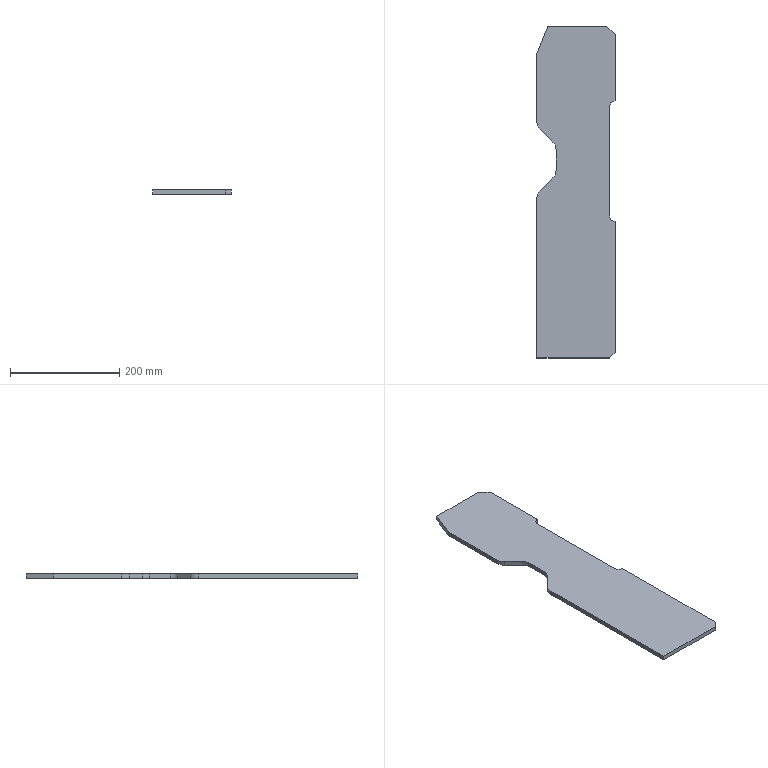Part | SolidWorks | features Extrusion 1 | 1 solid | 21 faces | box 143 x 607 x 8 mm | volume 646931 mm3 | plane 15 | cylinder 6 | commonest cylinder face diameters 40 x4 20 x2
STEP:
#1=CARTESIAN_POINT('',(0.,0.,0.));
#2=VERTEX_POINT('',#1);
#3=CARTESIAN_POINT('',(133.,0.,0.));
#4=VERTEX_POINT('',#3);
#5=CARTESIAN_POINT('',(133.,0.,0.));
#6=DIRECTION('',(1.,0.,0.));
#7=VECTOR('',#6,1000.);
#8=LINE('',#5,#7);
#9=EDGE_CURVE('',#2,#4,#8,.T.);
#10=ORIENTED_EDGE('',*,*,#9,.T.);
#11=CARTESIAN_POINT('',(133.,0.,8.));
#12=VERTEX_POINT('',#11);
#13=CARTESIAN_POINT('',(133.,0.,8.));
#14=DIRECTION('',(0.,0.,-1.));
#15=VECTOR('',#14,1000.);
#16=LINE('',#13,#15);
#17=EDGE_CURVE('',#12,#4,#16,.T.);
#18=ORIENTED_EDGE('',*,*,#17,.F.);
#19=CARTESIAN_POINT('',(0.,0.,8.));
#20=VERTEX_POINT('',#19);
#21=CARTESIAN_POINT('',(133.,0.,8.));
#22=DIRECTION('',(1.,0.,0.));
#23=VECTOR('',#22,1000.);
#24=LINE('',#21,#23);
#25=EDGE_CURVE('',#20,#12,#24,.T.);
#26=ORIENTED_EDGE('',*,*,#25,.F.);
#27=CARTESIAN_POINT('',(0.,0.,8.));
#28=DIRECTION('',(0.,0.,-1.));
#29=VECTOR('',#28,1000.);
#30=LINE('',#27,#29);
#31=EDGE_CURVE('',#20,#2,#30,.T.);
#32=ORIENTED_EDGE('',*,*,#31,.T.);
#33=EDGE_LOOP('',(#10,#18,#26,#32));
#34=FACE_OUTER_BOUND('',#33,.T.);
#35=CARTESIAN_POINT('',(133.,0.,8.));
#36=DIRECTION('',(0.,1.,0.));
#37=DIRECTION('',(0.,0.,1.));
#38=AXIS2_PLACEMENT_3D('',#35,#36,#37);
#39=PLANE('',#38);
#40=ADVANCED_FACE('',(#34),#39,.F.);
#41=CARTESIAN_POINT('',(143.,10.,0.));
#42=VERTEX_POINT('',#41);
#43=CARTESIAN_POINT('',(143.,10.,0.));
#44=DIRECTION('',(0.7071,0.7071,0.));
#45=VECTOR('',#44,1000.);
#46=LINE('',#43,#45);
#47=EDGE_CURVE('',#4,#42,#46,.T.);
#48=ORIENTED_EDGE('',*,*,#47,.T.);
#49=CARTESIAN_POINT('',(143.,10.,8.));
#50=VERTEX_POINT('',#49);
#51=CARTESIAN_POINT('',(143.,10.,8.));
#52=DIRECTION('',(0.,0.,-1.));
#53=VECTOR('',#52,1000.);
#54=LINE('',#51,#53);
#55=EDGE_CURVE('',#50,#42,#54,.T.);
#56=ORIENTED_EDGE('',*,*,#55,.F.);
#57=CARTESIAN_POINT('',(143.,10.,8.));
#58=DIRECTION('',(0.7071,0.7071,0.));
#59=VECTOR('',#58,1000.);
#60=LINE('',#57,#59);
#61=EDGE_CURVE('',#12,#50,#60,.T.);
#62=ORIENTED_EDGE('',*,*,#61,.F.);
#63=ORIENTED_EDGE('',*,*,#17,.T.);
#64=EDGE_LOOP('',(#48,#56,#62,#63));
#65=FACE_OUTER_BOUND('',#64,.T.);
#66=CARTESIAN_POINT('',(143.,10.,8.));
#67=DIRECTION('',(-0.7071,0.7071,0.));
#68=DIRECTION('',(-0.7071,-0.7071,0.));
#69=AXIS2_PLACEMENT_3D('',#66,#67,#68);
#70=PLANE('',#69);
#71=ADVANCED_FACE('',(#65),#70,.F.);
#72=CARTESIAN_POINT('',(143.,250.,0.));
#73=VERTEX_POINT('',#72);
#74=CARTESIAN_POINT('',(143.,250.,0.));
#75=DIRECTION('',(0.,1.,0.));
#76=VECTOR('',#75,1000.);
#77=LINE('',#74,#76);
#78=EDGE_CURVE('',#42,#73,#77,.T.);
#79=ORIENTED_EDGE('',*,*,#78,.T.);
#80=CARTESIAN_POINT('',(143.,250.,8.));
#81=VERTEX_POINT('',#80);
#82=CARTESIAN_POINT('',(143.,250.,8.));
#83=DIRECTION('',(0.,0.,-1.));
#84=VECTOR('',#83,1000.);
#85=LINE('',#82,#84);
#86=EDGE_CURVE('',#81,#73,#85,.T.);
#87=ORIENTED_EDGE('',*,*,#86,.F.);
#88=CARTESIAN_POINT('',(143.,250.,8.));
#89=DIRECTION('',(0.,1.,0.));
#90=VECTOR('',#89,1000.);
#91=LINE('',#88,#90);
#92=EDGE_CURVE('',#50,#81,#91,.T.);
#93=ORIENTED_EDGE('',*,*,#92,.F.);
#94=ORIENTED_EDGE('',*,*,#55,.T.);
#95=EDGE_LOOP('',(#79,#87,#93,#94));
#96=FACE_OUTER_BOUND('',#95,.T.);
#97=CARTESIAN_POINT('',(143.,250.,8.));
#98=DIRECTION('',(-1.,0.,0.));
#99=DIRECTION('',(0.,-1.,0.));
#100=AXIS2_PLACEMENT_3D('',#97,#98,#99);
#101=PLANE('',#100);
#102=ADVANCED_FACE('',(#96),#101,.F.);
#103=CARTESIAN_POINT('',(133.,260.,0.));
#104=VERTEX_POINT('',#103);
#105=CARTESIAN_POINT('',(143.,260.,0.));
#106=DIRECTION('',(0.,0.,-1.));
#107=DIRECTION('',(-1.,0.,0.));
#108=AXIS2_PLACEMENT_3D('',#105,#106,#107);
#109=CIRCLE('',#108,10.);
#110=EDGE_CURVE('',#73,#104,#109,.T.);
#111=ORIENTED_EDGE('',*,*,#110,.T.);
#112=CARTESIAN_POINT('',(133.,260.,8.));
#113=VERTEX_POINT('',#112);
#114=CARTESIAN_POINT('',(133.,260.,8.));
#115=DIRECTION('',(0.,0.,-1.));
#116=VECTOR('',#115,1000.);
#117=LINE('',#114,#116);
#118=EDGE_CURVE('',#113,#104,#117,.T.);
#119=ORIENTED_EDGE('',*,*,#118,.F.);
#120=CARTESIAN_POINT('',(143.,260.,8.));
#121=DIRECTION('',(0.,0.,-1.));
#122=DIRECTION('',(-1.,0.,0.));
#123=AXIS2_PLACEMENT_3D('',#120,#121,#122);
#124=CIRCLE('',#123,10.);
#125=EDGE_CURVE('',#81,#113,#124,.T.);
#126=ORIENTED_EDGE('',*,*,#125,.F.);
#127=ORIENTED_EDGE('',*,*,#86,.T.);
#128=EDGE_LOOP('',(#111,#119,#126,#127));
#129=FACE_OUTER_BOUND('',#128,.T.);
#130=CARTESIAN_POINT('',(143.,260.,8.));
#131=DIRECTION('',(0.,0.,-1.));
#132=DIRECTION('',(-1.,0.,0.));
#133=AXIS2_PLACEMENT_3D('',#130,#131,#132);
#134=CYLINDRICAL_SURFACE('',#133,10.);
#135=ADVANCED_FACE('',(#129),#134,.F.);
#136=CARTESIAN_POINT('',(133.,460.,0.));
#137=VERTEX_POINT('',#136);
#138=CARTESIAN_POINT('',(133.,460.,0.));
#139=DIRECTION('',(0.,1.,0.));
#140=VECTOR('',#139,1000.);
#141=LINE('',#138,#140);
#142=EDGE_CURVE('',#104,#137,#141,.T.);
#143=ORIENTED_EDGE('',*,*,#142,.T.);
#144=CARTESIAN_POINT('',(133.,460.,8.));
#145=VERTEX_POINT('',#144);
#146=CARTESIAN_POINT('',(133.,460.,8.));
#147=DIRECTION('',(0.,0.,-1.));
#148=VECTOR('',#147,1000.);
#149=LINE('',#146,#148);
#150=EDGE_CURVE('',#145,#137,#149,.T.);
#151=ORIENTED_EDGE('',*,*,#150,.F.);
#152=CARTESIAN_POINT('',(133.,460.,8.));
#153=DIRECTION('',(0.,1.,0.));
#154=VECTOR('',#153,1000.);
#155=LINE('',#152,#154);
#156=EDGE_CURVE('',#113,#145,#155,.T.);
#157=ORIENTED_EDGE('',*,*,#156,.F.);
#158=ORIENTED_EDGE('',*,*,#118,.T.);
#159=EDGE_LOOP('',(#143,#151,#157,#158));
#160=FACE_OUTER_BOUND('',#159,.T.);
#161=CARTESIAN_POINT('',(133.,460.,8.));
#162=DIRECTION('',(-1.,0.,0.));
#163=DIRECTION('',(0.,-1.,0.));
#164=AXIS2_PLACEMENT_3D('',#161,#162,#163);
#165=PLANE('',#164);
#166=ADVANCED_FACE('',(#160),#165,.F.);
#167=CARTESIAN_POINT('',(143.,470.,0.));
#168=VERTEX_POINT('',#167);
#169=CARTESIAN_POINT('',(143.,460.,0.));
#170=DIRECTION('',(0.,0.,-1.));
#171=DIRECTION('',(1.,0.,0.));
#172=AXIS2_PLACEMENT_3D('',#169,#170,#171);
#173=CIRCLE('',#172,10.);
#174=EDGE_CURVE('',#137,#168,#173,.T.);
#175=ORIENTED_EDGE('',*,*,#174,.T.);
#176=CARTESIAN_POINT('',(143.,470.,8.));
#177=VERTEX_POINT('',#176);
#178=CARTESIAN_POINT('',(143.,470.,8.));
#179=DIRECTION('',(0.,0.,-1.));
#180=VECTOR('',#179,1000.);
#181=LINE('',#178,#180);
#182=EDGE_CURVE('',#177,#168,#181,.T.);
#183=ORIENTED_EDGE('',*,*,#182,.F.);
#184=CARTESIAN_POINT('',(143.,460.,8.));
#185=DIRECTION('',(0.,0.,-1.));
#186=DIRECTION('',(1.,0.,0.));
#187=AXIS2_PLACEMENT_3D('',#184,#185,#186);
#188=CIRCLE('',#187,10.);
#189=EDGE_CURVE('',#145,#177,#188,.T.);
#190=ORIENTED_EDGE('',*,*,#189,.F.);
#191=ORIENTED_EDGE('',*,*,#150,.T.);
#192=EDGE_LOOP('',(#175,#183,#190,#191));
#193=FACE_OUTER_BOUND('',#192,.T.);
#194=CARTESIAN_POINT('',(143.,460.,8.));
#195=DIRECTION('',(0.,0.,-1.));
#196=DIRECTION('',(-1.,0.,0.));
#197=AXIS2_PLACEMENT_3D('',#194,#195,#196);
#198=CYLINDRICAL_SURFACE('',#197,10.);
#199=ADVANCED_FACE('',(#193),#198,.F.);
#200=CARTESIAN_POINT('',(143.,592.,0.));
#201=VERTEX_POINT('',#200);
#202=CARTESIAN_POINT('',(143.,592.,0.));
#203=DIRECTION('',(0.,1.,0.));
#204=VECTOR('',#203,1000.);
#205=LINE('',#202,#204);
#206=EDGE_CURVE('',#168,#201,#205,.T.);
#207=ORIENTED_EDGE('',*,*,#206,.T.);
#208=CARTESIAN_POINT('',(143.,592.,8.));
#209=VERTEX_POINT('',#208);
#210=CARTESIAN_POINT('',(143.,592.,8.));
#211=DIRECTION('',(0.,0.,-1.));
#212=VECTOR('',#211,1000.);
#213=LINE('',#210,#212);
#214=EDGE_CURVE('',#209,#201,#213,.T.);
#215=ORIENTED_EDGE('',*,*,#214,.F.);
#216=CARTESIAN_POINT('',(143.,592.,8.));
#217=DIRECTION('',(0.,1.,0.));
#218=VECTOR('',#217,1000.);
#219=LINE('',#216,#218);
#220=EDGE_CURVE('',#177,#209,#219,.T.);
#221=ORIENTED_EDGE('',*,*,#220,.F.);
#222=ORIENTED_EDGE('',*,*,#182,.T.);
#223=EDGE_LOOP('',(#207,#215,#221,#222));
#224=FACE_OUTER_BOUND('',#223,.T.);
#225=CARTESIAN_POINT('',(143.,592.,8.));
#226=DIRECTION('',(-1.,0.,0.));
#227=DIRECTION('',(0.,0.,1.));
#228=AXIS2_PLACEMENT_3D('',#225,#226,#227);
#229=PLANE('',#228);
#230=ADVANCED_FACE('',(#224),#229,.F.);
#231=CARTESIAN_POINT('',(128.,607.,0.));
#232=VERTEX_POINT('',#231);
#233=CARTESIAN_POINT('',(128.,607.,0.));
#234=DIRECTION('',(-0.7071,0.7071,0.));
#235=VECTOR('',#234,1000.);
#236=LINE('',#233,#235);
#237=EDGE_CURVE('',#201,#232,#236,.T.);
#238=ORIENTED_EDGE('',*,*,#237,.T.);
#239=CARTESIAN_POINT('',(128.,607.,8.));
#240=VERTEX_POINT('',#239);
#241=CARTESIAN_POINT('',(128.,607.,8.));
#242=DIRECTION('',(0.,0.,-1.));
#243=VECTOR('',#242,1000.);
#244=LINE('',#241,#243);
#245=EDGE_CURVE('',#240,#232,#244,.T.);
#246=ORIENTED_EDGE('',*,*,#245,.F.);
#247=CARTESIAN_POINT('',(128.,607.,8.));
#248=DIRECTION('',(-0.7071,0.7071,0.));
#249=VECTOR('',#248,1000.);
#250=LINE('',#247,#249);
#251=EDGE_CURVE('',#209,#240,#250,.T.);
#252=ORIENTED_EDGE('',*,*,#251,.F.);
#253=ORIENTED_EDGE('',*,*,#214,.T.);
#254=EDGE_LOOP('',(#238,#246,#252,#253));
#255=FACE_OUTER_BOUND('',#254,.T.);
#256=CARTESIAN_POINT('',(128.,607.,8.));
#257=DIRECTION('',(-0.7071,-0.7071,0.));
#258=DIRECTION('',(0.7071,-0.7071,0.));
#259=AXIS2_PLACEMENT_3D('',#256,#257,#258);
#260=PLANE('',#259);
#261=ADVANCED_FACE('',(#255),#260,.F.);
#262=CARTESIAN_POINT('',(20.,607.,0.));
#263=VERTEX_POINT('',#262);
#264=CARTESIAN_POINT('',(20.,607.,0.));
#265=DIRECTION('',(-1.,0.,0.));
#266=VECTOR('',#265,1000.);
#267=LINE('',#264,#266);
#268=EDGE_CURVE('',#232,#263,#267,.T.);
#269=ORIENTED_EDGE('',*,*,#268,.T.);
#270=CARTESIAN_POINT('',(20.,607.,8.));
#271=VERTEX_POINT('',#270);
#272=CARTESIAN_POINT('',(20.,607.,8.));
#273=DIRECTION('',(0.,0.,-1.));
#274=VECTOR('',#273,1000.);
#275=LINE('',#272,#274);
#276=EDGE_CURVE('',#271,#263,#275,.T.);
#277=ORIENTED_EDGE('',*,*,#276,.F.);
#278=CARTESIAN_POINT('',(20.,607.,8.));
#279=DIRECTION('',(-1.,0.,0.));
#280=VECTOR('',#279,1000.);
#281=LINE('',#278,#280);
#282=EDGE_CURVE('',#240,#271,#281,.T.);
#283=ORIENTED_EDGE('',*,*,#282,.F.);
#284=ORIENTED_EDGE('',*,*,#245,.T.);
#285=EDGE_LOOP('',(#269,#277,#283,#284));
#286=FACE_OUTER_BOUND('',#285,.T.);
#287=CARTESIAN_POINT('',(20.,607.,8.));
#288=DIRECTION('',(0.,-1.,0.));
#289=DIRECTION('',(0.,0.,-1.));
#290=AXIS2_PLACEMENT_3D('',#287,#288,#289);
#291=PLANE('',#290);
#292=ADVANCED_FACE('',(#286),#291,.F.);
#293=CARTESIAN_POINT('',(0.,557.,0.));
#294=VERTEX_POINT('',#293);
#295=CARTESIAN_POINT('',(0.,557.,0.));
#296=DIRECTION('',(-0.3714,-0.9285,0.));
#297=VECTOR('',#296,1000.);
#298=LINE('',#295,#297);
#299=EDGE_CURVE('',#263,#294,#298,.T.);
#300=ORIENTED_EDGE('',*,*,#299,.T.);
#301=CARTESIAN_POINT('',(0.,557.,8.));
#302=VERTEX_POINT('',#301);
#303=CARTESIAN_POINT('',(0.,557.,8.));
#304=DIRECTION('',(0.,0.,-1.));
#305=VECTOR('',#304,1000.);
#306=LINE('',#303,#305);
#307=EDGE_CURVE('',#302,#294,#306,.T.);
#308=ORIENTED_EDGE('',*,*,#307,.F.);
#309=CARTESIAN_POINT('',(0.,557.,8.));
#310=DIRECTION('',(-0.3714,-0.9285,0.));
#311=VECTOR('',#310,1000.);
#312=LINE('',#309,#311);
#313=EDGE_CURVE('',#271,#302,#312,.T.);
#314=ORIENTED_EDGE('',*,*,#313,.F.);
#315=ORIENTED_EDGE('',*,*,#276,.T.);
#316=EDGE_LOOP('',(#300,#308,#314,#315));
#317=FACE_OUTER_BOUND('',#316,.T.);
#318=CARTESIAN_POINT('',(0.,557.,8.));
#319=DIRECTION('',(0.9285,-0.3714,0.));
#320=DIRECTION('',(0.3714,0.9285,0.));
#321=AXIS2_PLACEMENT_3D('',#318,#319,#320);
#322=PLANE('',#321);
#323=ADVANCED_FACE('',(#317),#322,.F.);
#324=CARTESIAN_POINT('',(0.,432.284,0.));
#325=VERTEX_POINT('',#324);
#326=CARTESIAN_POINT('',(0.,432.284,0.));
#327=DIRECTION('',(0.,-1.,0.));
#328=VECTOR('',#327,1000.);
#329=LINE('',#326,#328);
#330=EDGE_CURVE('',#294,#325,#329,.T.);
#331=ORIENTED_EDGE('',*,*,#330,.T.);
#332=CARTESIAN_POINT('',(0.,432.284,8.));
#333=VERTEX_POINT('',#332);
#334=CARTESIAN_POINT('',(0.,432.284,8.));
#335=DIRECTION('',(0.,0.,-1.));
#336=VECTOR('',#335,1000.);
#337=LINE('',#334,#336);
#338=EDGE_CURVE('',#333,#325,#337,.T.);
#339=ORIENTED_EDGE('',*,*,#338,.F.);
#340=CARTESIAN_POINT('',(0.,432.284,8.));
#341=DIRECTION('',(0.,-1.,0.));
#342=VECTOR('',#341,1000.);
#343=LINE('',#340,#342);
#344=EDGE_CURVE('',#302,#333,#343,.T.);
#345=ORIENTED_EDGE('',*,*,#344,.F.);
#346=ORIENTED_EDGE('',*,*,#307,.T.);
#347=EDGE_LOOP('',(#331,#339,#345,#346));
#348=FACE_OUTER_BOUND('',#347,.T.);
#349=CARTESIAN_POINT('',(0.,432.284,8.));
#350=DIRECTION('',(1.,0.,0.));
#351=DIRECTION('',(0.,0.,-1.));
#352=AXIS2_PLACEMENT_3D('',#349,#350,#351);
#353=PLANE('',#352);
#354=ADVANCED_FACE('',(#348),#353,.F.);
#355=CARTESIAN_POINT('',(5.858,418.142,0.));
#356=VERTEX_POINT('',#355);
#357=CARTESIAN_POINT('',(20.,432.284,0.));
#358=DIRECTION('',(0.,0.,1.));
#359=DIRECTION('',(-1.,0.,0.));
#360=AXIS2_PLACEMENT_3D('',#357,#358,#359);
#361=CIRCLE('',#360,20.);
#362=EDGE_CURVE('',#325,#356,#361,.T.);
#363=ORIENTED_EDGE('',*,*,#362,.T.);
#364=CARTESIAN_POINT('',(5.858,418.142,8.));
#365=VERTEX_POINT('',#364);
#366=CARTESIAN_POINT('',(5.858,418.142,8.));
#367=DIRECTION('',(0.,0.,-1.));
#368=VECTOR('',#367,1000.);
#369=LINE('',#366,#368);
#370=EDGE_CURVE('',#365,#356,#369,.T.);
#371=ORIENTED_EDGE('',*,*,#370,.F.);
#372=CARTESIAN_POINT('',(20.,432.284,8.));
#373=DIRECTION('',(0.,0.,1.));
#374=DIRECTION('',(-1.,0.,0.));
#375=AXIS2_PLACEMENT_3D('',#372,#373,#374);
#376=CIRCLE('',#375,20.);
#377=EDGE_CURVE('',#333,#365,#376,.T.);
#378=ORIENTED_EDGE('',*,*,#377,.F.);
#379=ORIENTED_EDGE('',*,*,#338,.T.);
#380=EDGE_LOOP('',(#363,#371,#378,#379));
#381=FACE_OUTER_BOUND('',#380,.T.);
#382=CARTESIAN_POINT('',(20.,432.284,8.));
#383=DIRECTION('',(0.,0.,-1.));
#384=DIRECTION('',(-1.,0.,0.));
#385=AXIS2_PLACEMENT_3D('',#382,#383,#384);
#386=CYLINDRICAL_SURFACE('',#385,20.);
#387=ADVANCED_FACE('',(#381),#386,.T.);
#388=CARTESIAN_POINT('',(29.142,394.858,0.));
#389=VERTEX_POINT('',#388);
#390=CARTESIAN_POINT('',(29.142,394.858,0.));
#391=DIRECTION('',(0.7071,-0.7071,0.));
#392=VECTOR('',#391,1000.);
#393=LINE('',#390,#392);
#394=EDGE_CURVE('',#356,#389,#393,.T.);
#395=ORIENTED_EDGE('',*,*,#394,.T.);
#396=CARTESIAN_POINT('',(29.142,394.858,8.));
#397=VERTEX_POINT('',#396);
#398=CARTESIAN_POINT('',(29.142,394.858,8.));
#399=DIRECTION('',(0.,0.,-1.));
#400=VECTOR('',#399,1000.);
#401=LINE('',#398,#400);
#402=EDGE_CURVE('',#397,#389,#401,.T.);
#403=ORIENTED_EDGE('',*,*,#402,.F.);
#404=CARTESIAN_POINT('',(29.142,394.858,8.));
#405=DIRECTION('',(0.7071,-0.7071,0.));
#406=VECTOR('',#405,1000.);
#407=LINE('',#404,#406);
#408=EDGE_CURVE('',#365,#397,#407,.T.);
#409=ORIENTED_EDGE('',*,*,#408,.F.);
#410=ORIENTED_EDGE('',*,*,#370,.T.);
#411=EDGE_LOOP('',(#395,#403,#409,#410));
#412=FACE_OUTER_BOUND('',#411,.T.);
#413=CARTESIAN_POINT('',(29.142,394.858,8.));
#414=DIRECTION('',(0.7071,0.7071,0.));
#415=DIRECTION('',(-0.7071,0.7071,0.));
#416=AXIS2_PLACEMENT_3D('',#413,#414,#415);
#417=PLANE('',#416);
#418=ADVANCED_FACE('',(#412),#417,.F.);
#419=CARTESIAN_POINT('',(35.,380.716,0.));
#420=VERTEX_POINT('',#419);
#421=CARTESIAN_POINT('',(15.,380.716,0.));
#422=DIRECTION('',(0.,0.,-1.));
#423=DIRECTION('',(1.,0.,0.));
#424=AXIS2_PLACEMENT_3D('',#421,#422,#423);
#425=CIRCLE('',#424,20.);
#426=EDGE_CURVE('',#389,#420,#425,.T.);
#427=ORIENTED_EDGE('',*,*,#426,.T.);
#428=CARTESIAN_POINT('',(35.,380.716,8.));
#429=VERTEX_POINT('',#428);
#430=CARTESIAN_POINT('',(35.,380.716,8.));
#431=DIRECTION('',(0.,0.,-1.));
#432=VECTOR('',#431,1000.);
#433=LINE('',#430,#432);
#434=EDGE_CURVE('',#429,#420,#433,.T.);
#435=ORIENTED_EDGE('',*,*,#434,.F.);
#436=CARTESIAN_POINT('',(15.,380.716,8.));
#437=DIRECTION('',(0.,0.,-1.));
#438=DIRECTION('',(1.,0.,0.));
#439=AXIS2_PLACEMENT_3D('',#436,#437,#438);
#440=CIRCLE('',#439,20.);
#441=EDGE_CURVE('',#397,#429,#440,.T.);
#442=ORIENTED_EDGE('',*,*,#441,.F.);
#443=ORIENTED_EDGE('',*,*,#402,.T.);
#444=EDGE_LOOP('',(#427,#435,#442,#443));
#445=FACE_OUTER_BOUND('',#444,.T.);
#446=CARTESIAN_POINT('',(15.,380.716,8.));
#447=DIRECTION('',(0.,0.,-1.));
#448=DIRECTION('',(-1.,0.,0.));
#449=AXIS2_PLACEMENT_3D('',#446,#447,#448);
#450=CYLINDRICAL_SURFACE('',#449,20.);
#451=ADVANCED_FACE('',(#445),#450,.F.);
#452=CARTESIAN_POINT('',(35.,343.284,0.));
#453=VERTEX_POINT('',#452);
#454=CARTESIAN_POINT('',(35.,343.284,0.));
#455=DIRECTION('',(0.,-1.,0.));
#456=VECTOR('',#455,1000.);
#457=LINE('',#454,#456);
#458=EDGE_CURVE('',#420,#453,#457,.T.);
#459=ORIENTED_EDGE('',*,*,#458,.T.);
#460=CARTESIAN_POINT('',(35.,343.284,8.));
#461=VERTEX_POINT('',#460);
#462=CARTESIAN_POINT('',(35.,343.284,8.));
#463=DIRECTION('',(0.,0.,-1.));
#464=VECTOR('',#463,1000.);
#465=LINE('',#462,#464);
#466=EDGE_CURVE('',#461,#453,#465,.T.);
#467=ORIENTED_EDGE('',*,*,#466,.F.);
#468=CARTESIAN_POINT('',(35.,343.284,8.));
#469=DIRECTION('',(0.,-1.,0.));
#470=VECTOR('',#469,1000.);
#471=LINE('',#468,#470);
#472=EDGE_CURVE('',#429,#461,#471,.T.);
#473=ORIENTED_EDGE('',*,*,#472,.F.);
#474=ORIENTED_EDGE('',*,*,#434,.T.);
#475=EDGE_LOOP('',(#459,#467,#473,#474));
#476=FACE_OUTER_BOUND('',#475,.T.);
#477=CARTESIAN_POINT('',(35.,343.284,8.));
#478=DIRECTION('',(1.,0.,0.));
#479=DIRECTION('',(0.,1.,0.));
#480=AXIS2_PLACEMENT_3D('',#477,#478,#479);
#481=PLANE('',#480);
#482=ADVANCED_FACE('',(#476),#481,.F.);
#483=CARTESIAN_POINT('',(29.142,329.142,0.));
#484=VERTEX_POINT('',#483);
#485=CARTESIAN_POINT('',(15.,343.284,0.));
#486=DIRECTION('',(0.,0.,-1.));
#487=DIRECTION('',(1.,0.,0.));
#488=AXIS2_PLACEMENT_3D('',#485,#486,#487);
#489=CIRCLE('',#488,20.);
#490=EDGE_CURVE('',#453,#484,#489,.T.);
#491=ORIENTED_EDGE('',*,*,#490,.T.);
#492=CARTESIAN_POINT('',(29.142,329.142,8.));
#493=VERTEX_POINT('',#492);
#494=CARTESIAN_POINT('',(29.142,329.142,8.));
#495=DIRECTION('',(0.,0.,-1.));
#496=VECTOR('',#495,1000.);
#497=LINE('',#494,#496);
#498=EDGE_CURVE('',#493,#484,#497,.T.);
#499=ORIENTED_EDGE('',*,*,#498,.F.);
#500=CARTESIAN_POINT('',(15.,343.284,8.));
#501=DIRECTION('',(0.,0.,-1.));
#502=DIRECTION('',(1.,0.,0.));
#503=AXIS2_PLACEMENT_3D('',#500,#501,#502);
#504=CIRCLE('',#503,20.);
#505=EDGE_CURVE('',#461,#493,#504,.T.);
#506=ORIENTED_EDGE('',*,*,#505,.F.);
#507=ORIENTED_EDGE('',*,*,#466,.T.);
#508=EDGE_LOOP('',(#491,#499,#506,#507));
#509=FACE_OUTER_BOUND('',#508,.T.);
#510=CARTESIAN_POINT('',(15.,343.284,8.));
#511=DIRECTION('',(0.,0.,-1.));
#512=DIRECTION('',(-1.,0.,0.));
#513=AXIS2_PLACEMENT_3D('',#510,#511,#512);
#514=CYLINDRICAL_SURFACE('',#513,20.);
#515=ADVANCED_FACE('',(#509),#514,.F.);
#516=CARTESIAN_POINT('',(5.858,305.858,0.));
#517=VERTEX_POINT('',#516);
#518=CARTESIAN_POINT('',(5.858,305.858,0.));
#519=DIRECTION('',(-0.7071,-0.7071,0.));
#520=VECTOR('',#519,1000.);
#521=LINE('',#518,#520);
#522=EDGE_CURVE('',#484,#517,#521,.T.);
#523=ORIENTED_EDGE('',*,*,#522,.T.);
#524=CARTESIAN_POINT('',(5.858,305.858,8.));
#525=VERTEX_POINT('',#524);
#526=CARTESIAN_POINT('',(5.858,305.858,8.));
#527=DIRECTION('',(0.,0.,-1.));
#528=VECTOR('',#527,1000.);
#529=LINE('',#526,#528);
#530=EDGE_CURVE('',#525,#517,#529,.T.);
#531=ORIENTED_EDGE('',*,*,#530,.F.);
#532=CARTESIAN_POINT('',(5.858,305.858,8.));
#533=DIRECTION('',(-0.7071,-0.7071,0.));
#534=VECTOR('',#533,1000.);
#535=LINE('',#532,#534);
#536=EDGE_CURVE('',#493,#525,#535,.T.);
#537=ORIENTED_EDGE('',*,*,#536,.F.);
#538=ORIENTED_EDGE('',*,*,#498,.T.);
#539=EDGE_LOOP('',(#523,#531,#537,#538));
#540=FACE_OUTER_BOUND('',#539,.T.);
#541=CARTESIAN_POINT('',(5.858,305.858,8.));
#542=DIRECTION('',(0.7071,-0.7071,0.));
#543=DIRECTION('',(0.7071,0.7071,0.));
#544=AXIS2_PLACEMENT_3D('',#541,#542,#543);
#545=PLANE('',#544);
#546=ADVANCED_FACE('',(#540),#545,.F.);
#547=CARTESIAN_POINT('',(0.,291.716,0.));
#548=VERTEX_POINT('',#547);
#549=CARTESIAN_POINT('',(20.,291.716,0.));
#550=DIRECTION('',(0.,0.,1.));
#551=DIRECTION('',(-1.,0.,0.));
#552=AXIS2_PLACEMENT_3D('',#549,#550,#551);
#553=CIRCLE('',#552,20.);
#554=EDGE_CURVE('',#517,#548,#553,.T.);
#555=ORIENTED_EDGE('',*,*,#554,.T.);
#556=CARTESIAN_POINT('',(0.,291.716,8.));
#557=VERTEX_POINT('',#556);
#558=CARTESIAN_POINT('',(0.,291.716,8.));
#559=DIRECTION('',(0.,0.,-1.));
#560=VECTOR('',#559,1000.);
#561=LINE('',#558,#560);
#562=EDGE_CURVE('',#557,#548,#561,.T.);
#563=ORIENTED_EDGE('',*,*,#562,.F.);
#564=CARTESIAN_POINT('',(20.,291.716,8.));
#565=DIRECTION('',(0.,0.,1.));
#566=DIRECTION('',(-1.,0.,0.));
#567=AXIS2_PLACEMENT_3D('',#564,#565,#566);
#568=CIRCLE('',#567,20.);
#569=EDGE_CURVE('',#525,#557,#568,.T.);
#570=ORIENTED_EDGE('',*,*,#569,.F.);
#571=ORIENTED_EDGE('',*,*,#530,.T.);
#572=EDGE_LOOP('',(#555,#563,#570,#571));
#573=FACE_OUTER_BOUND('',#572,.T.);
#574=CARTESIAN_POINT('',(20.,291.716,8.));
#575=DIRECTION('',(0.,0.,-1.));
#576=DIRECTION('',(-1.,0.,0.));
#577=AXIS2_PLACEMENT_3D('',#574,#575,#576);
#578=CYLINDRICAL_SURFACE('',#577,20.);
#579=ADVANCED_FACE('',(#573),#578,.T.);
#580=CARTESIAN_POINT('',(0.,0.,0.));
#581=DIRECTION('',(0.,-1.,0.));
#582=VECTOR('',#581,1000.);
#583=LINE('',#580,#582);
#584=EDGE_CURVE('',#548,#2,#583,.T.);
#585=ORIENTED_EDGE('',*,*,#584,.T.);
#586=ORIENTED_EDGE('',*,*,#31,.F.);
#587=CARTESIAN_POINT('',(0.,0.,8.));
#588=DIRECTION('',(0.,-1.,0.));
#589=VECTOR('',#588,1000.);
#590=LINE('',#587,#589);
#591=EDGE_CURVE('',#557,#20,#590,.T.);
#592=ORIENTED_EDGE('',*,*,#591,.F.);
#593=ORIENTED_EDGE('',*,*,#562,.T.);
#594=EDGE_LOOP('',(#585,#586,#592,#593));
#595=FACE_OUTER_BOUND('',#594,.T.);
#596=CARTESIAN_POINT('',(0.,0.,8.));
#597=DIRECTION('',(1.,0.,0.));
#598=DIRECTION('',(0.,0.,-1.));
#599=AXIS2_PLACEMENT_3D('',#596,#597,#598);
#600=PLANE('',#599);
#601=ADVANCED_FACE('',(#595),#600,.F.);
#602=ORIENTED_EDGE('',*,*,#25,.T.);
#603=ORIENTED_EDGE('',*,*,#61,.T.);
#604=ORIENTED_EDGE('',*,*,#92,.T.);
#605=ORIENTED_EDGE('',*,*,#125,.T.);
#606=ORIENTED_EDGE('',*,*,#156,.T.);
#607=ORIENTED_EDGE('',*,*,#189,.T.);
#608=ORIENTED_EDGE('',*,*,#220,.T.);
#609=ORIENTED_EDGE('',*,*,#251,.T.);
#610=ORIENTED_EDGE('',*,*,#282,.T.);
#611=ORIENTED_EDGE('',*,*,#313,.T.);
#612=ORIENTED_EDGE('',*,*,#344,.T.);
#613=ORIENTED_EDGE('',*,*,#377,.T.);
#614=ORIENTED_EDGE('',*,*,#408,.T.);
#615=ORIENTED_EDGE('',*,*,#441,.T.);
#616=ORIENTED_EDGE('',*,*,#472,.T.);
#617=ORIENTED_EDGE('',*,*,#505,.T.);
#618=ORIENTED_EDGE('',*,*,#536,.T.);
#619=ORIENTED_EDGE('',*,*,#569,.T.);
#620=ORIENTED_EDGE('',*,*,#591,.T.);
#621=EDGE_LOOP('',(#602,#603,#604,#605,#606,#607,#608,#609,#610,#611,#612,#613,#614,#615,#616,#617,#618,#619,#620));
#622=FACE_OUTER_BOUND('',#621,.T.);
#623=CARTESIAN_POINT('',(20.,291.716,8.));
#624=DIRECTION('',(0.,0.,-1.));
#625=DIRECTION('',(-1.,0.,0.));
#626=AXIS2_PLACEMENT_3D('',#623,#624,#625);
#627=PLANE('',#626);
#628=ADVANCED_FACE('',(#622),#627,.F.);
#629=ORIENTED_EDGE('',*,*,#9,.F.);
#630=ORIENTED_EDGE('',*,*,#584,.F.);
#631=ORIENTED_EDGE('',*,*,#554,.F.);
#632=ORIENTED_EDGE('',*,*,#522,.F.);
#633=ORIENTED_EDGE('',*,*,#490,.F.);
#634=ORIENTED_EDGE('',*,*,#458,.F.);
#635=ORIENTED_EDGE('',*,*,#426,.F.);
#636=ORIENTED_EDGE('',*,*,#394,.F.);
#637=ORIENTED_EDGE('',*,*,#362,.F.);
#638=ORIENTED_EDGE('',*,*,#330,.F.);
#639=ORIENTED_EDGE('',*,*,#299,.F.);
#640=ORIENTED_EDGE('',*,*,#268,.F.);
#641=ORIENTED_EDGE('',*,*,#237,.F.);
#642=ORIENTED_EDGE('',*,*,#206,.F.);
#643=ORIENTED_EDGE('',*,*,#174,.F.);
#644=ORIENTED_EDGE('',*,*,#142,.F.);
#645=ORIENTED_EDGE('',*,*,#110,.F.);
#646=ORIENTED_EDGE('',*,*,#78,.F.);
#647=ORIENTED_EDGE('',*,*,#47,.F.);
#648=EDGE_LOOP('',(#629,#630,#631,#632,#633,#634,#635,#636,#637,#638,#639,#640,#641,#642,#643,#644,#645,#646,#647));
#649=FACE_OUTER_BOUND('',#648,.T.);
#650=CARTESIAN_POINT('',(20.,291.716,0.));
#651=DIRECTION('',(0.,0.,-1.));
#652=DIRECTION('',(-1.,0.,0.));
#653=AXIS2_PLACEMENT_3D('',#650,#651,#652);
#654=PLANE('',#653);
#655=ADVANCED_FACE('',(#649),#654,.T.);
#656=CLOSED_SHELL('',(#40,#71,#102,#135,#166,#199,#230,#261,#292,#323,#354,#387,#418,#451,#482,#515,#546,#579,#601,#628,#655));
#657=MANIFOLD_SOLID_BREP('',#656);
#658=CARTESIAN_POINT('',(0.,0.,0.));
#659=DIRECTION('',(0.,0.,1.));
#660=DIRECTION('',(1.,0.,0.));
#661=AXIS2_PLACEMENT_3D('',#658,#659,#660);
#662=(LENGTH_UNIT()NAMED_UNIT(*)SI_UNIT(.MILLI.,.METRE.));
#663=UNCERTAINTY_MEASURE_WITH_UNIT(LENGTH_MEASURE(0.00001),#662,'','');
#664=(NAMED_UNIT(*)PLANE_ANGLE_UNIT()SI_UNIT($,.RADIAN.));
#665=(NAMED_UNIT(*)SI_UNIT($,.STERADIAN.)SOLID_ANGLE_UNIT());
#666=(GEOMETRIC_REPRESENTATION_CONTEXT(3)GLOBAL_UNCERTAINTY_ASSIGNED_CONTEXT((#663))GLOBAL_UNIT_ASSIGNED_CONTEXT((#662,#664,#665))REPRESENTATION_CONTEXT('',''));
#667=ADVANCED_BREP_SHAPE_REPRESENTATION('',(#657,#661),#666);